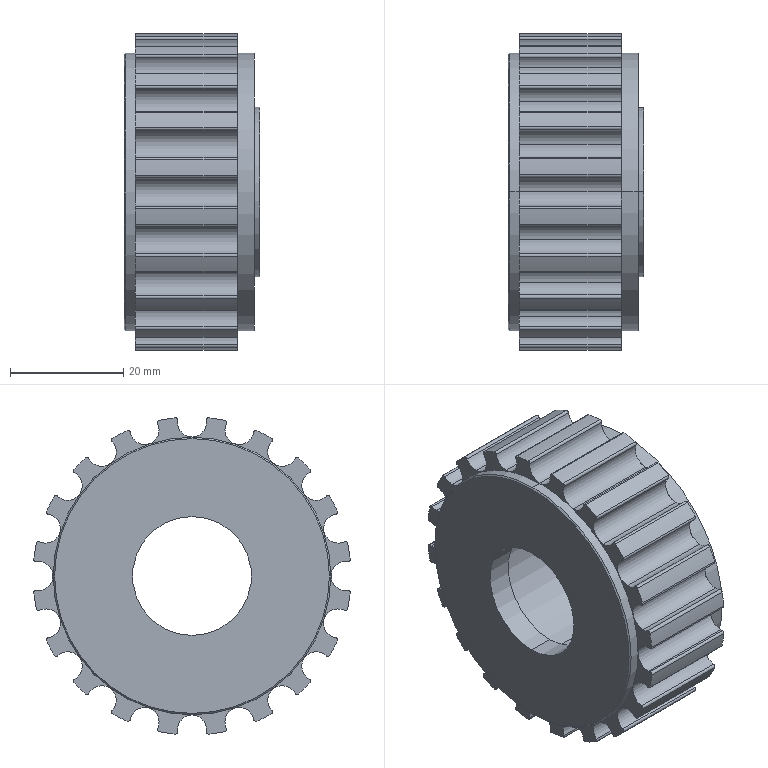Part | SolidWorks | features Chamfer 1, CirPattern 1, ICE 1, Revolution 1 | 1 solid | 129 faces | box 24 x 55.847 x 55.847 mm | volume 37187 mm3 | cylinder 119 | plane 8 | cone 2 | commonest cylinder face diameters 0.8 x52 5.14 x33 56.16 x20 26 x4 49 x4 21 x2